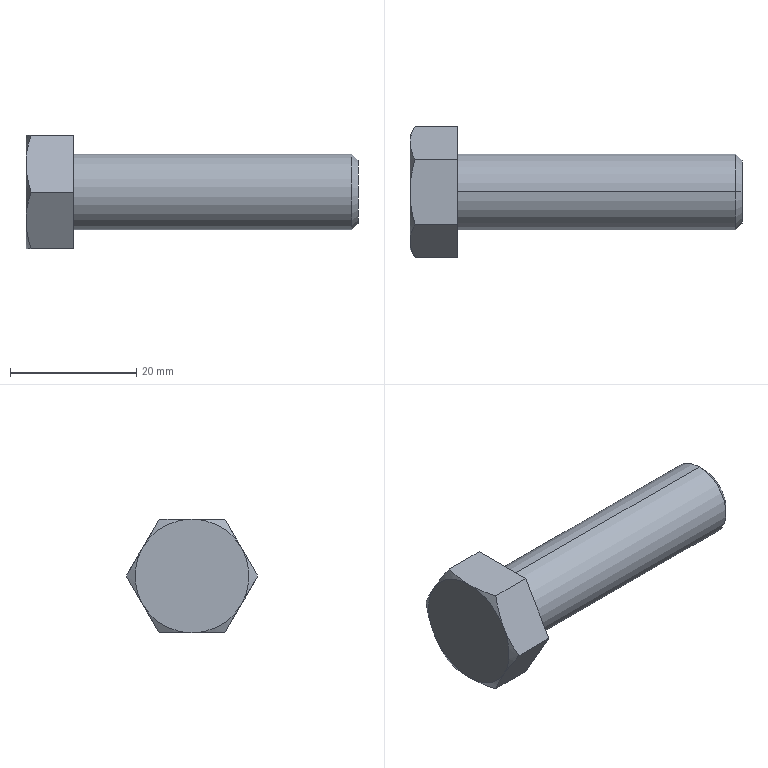Part | STEP file | hex bolt gradeb_bsi_BS EN 24015 - M12 x 45 x 30-N | 1 solid | 19 faces | box 52.5 x 20.785 x 18 mm | volume 7171 mm3 | plane 9 | cone 8 | cylinder 2 | commonest cylinder face diameters 12 x2